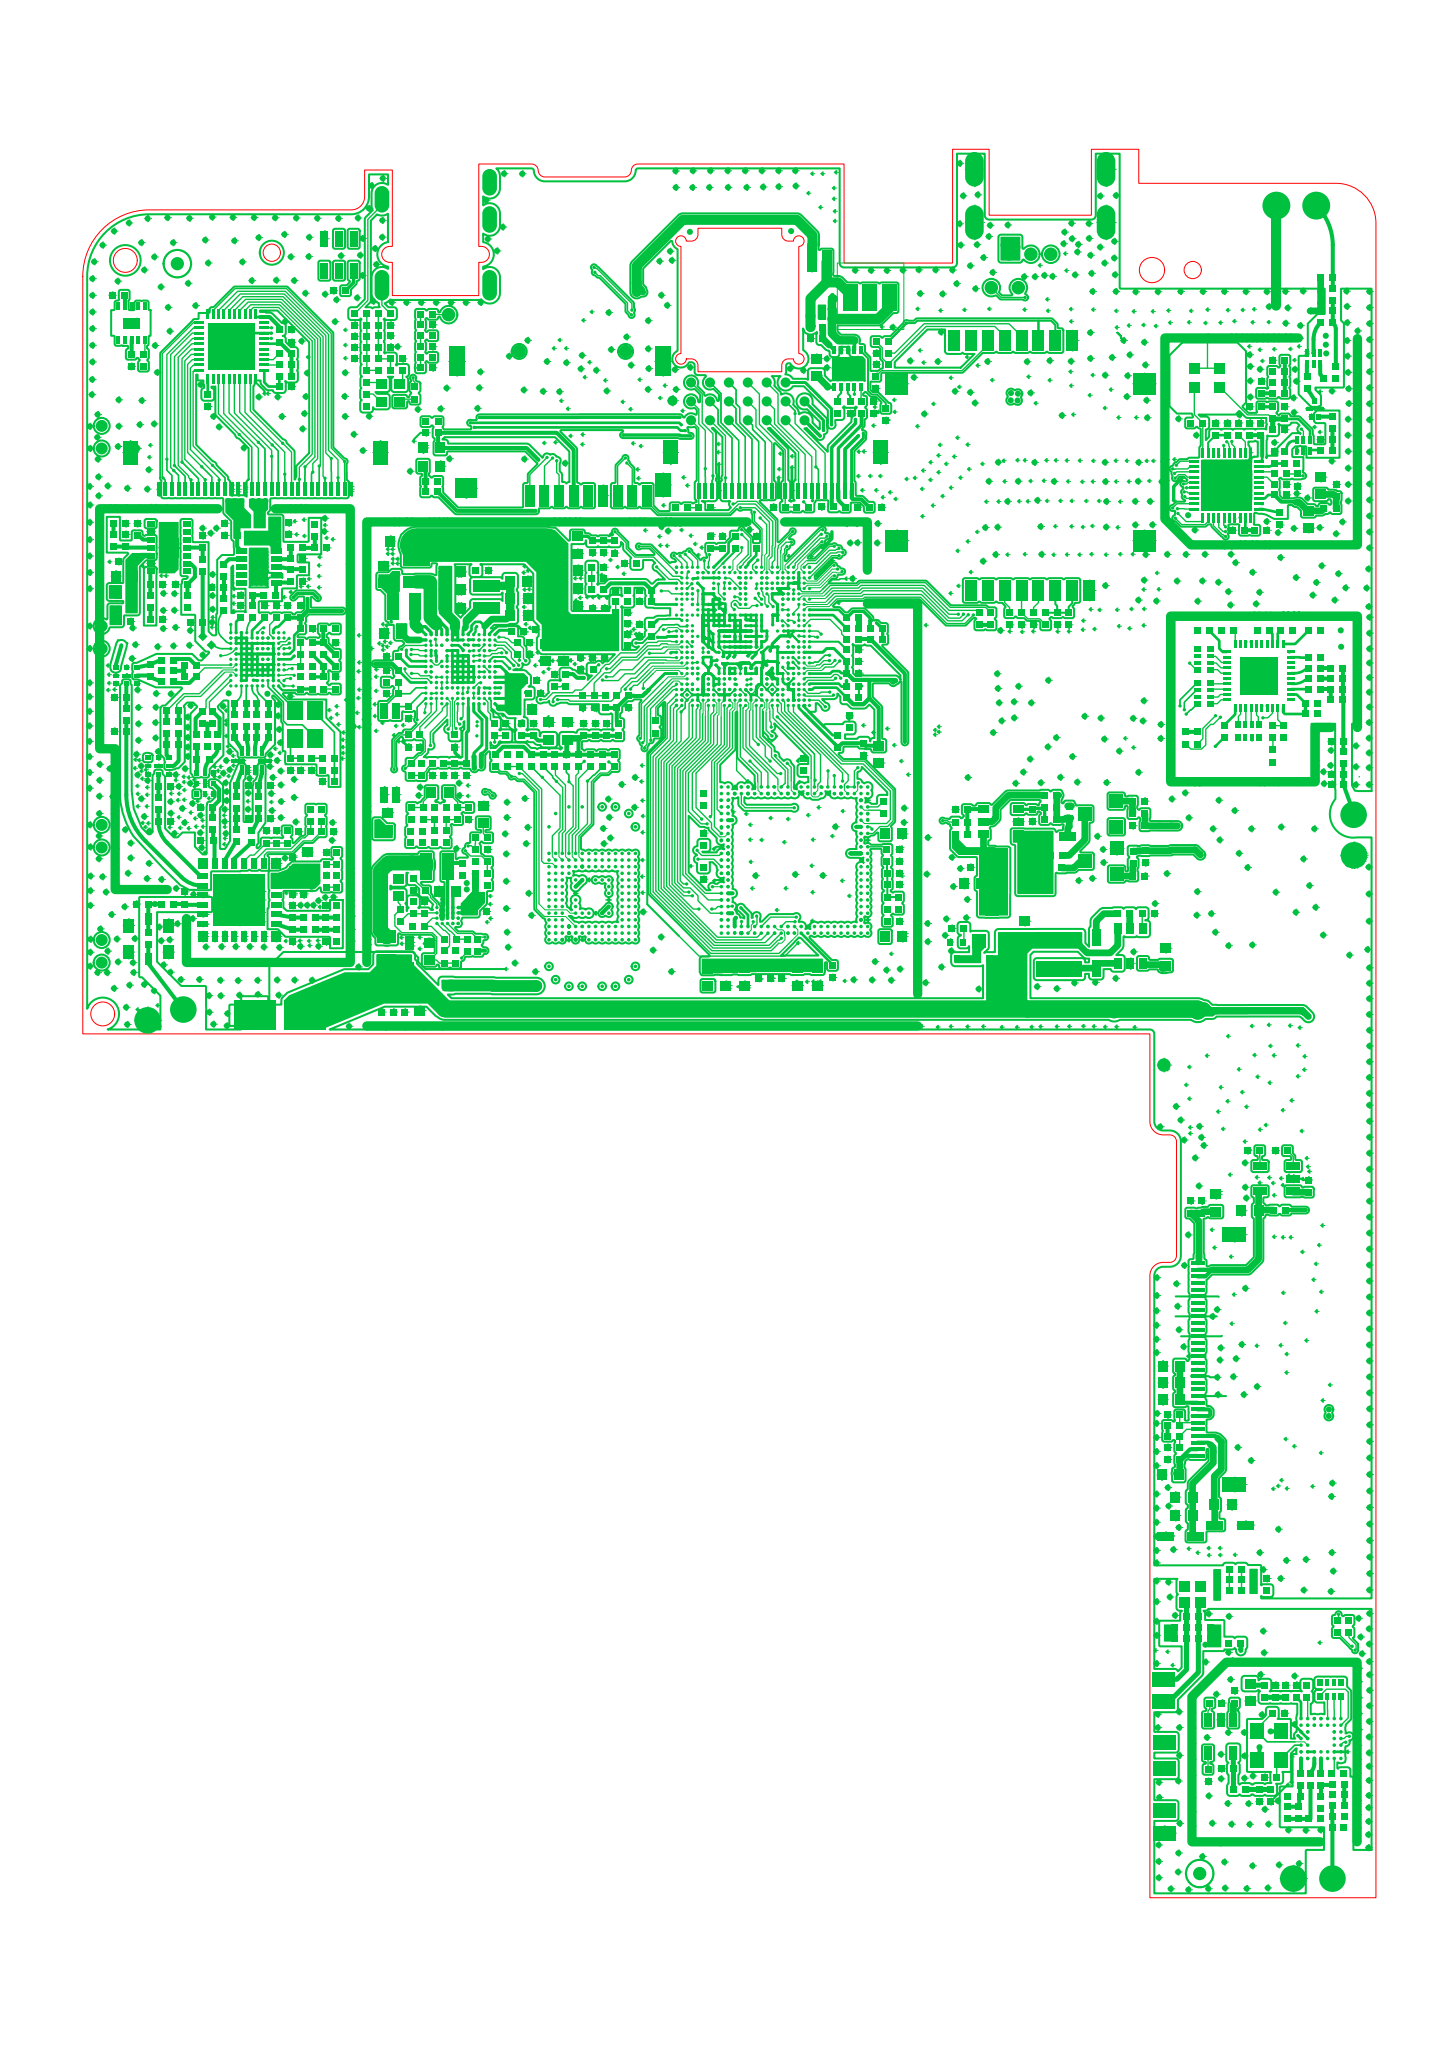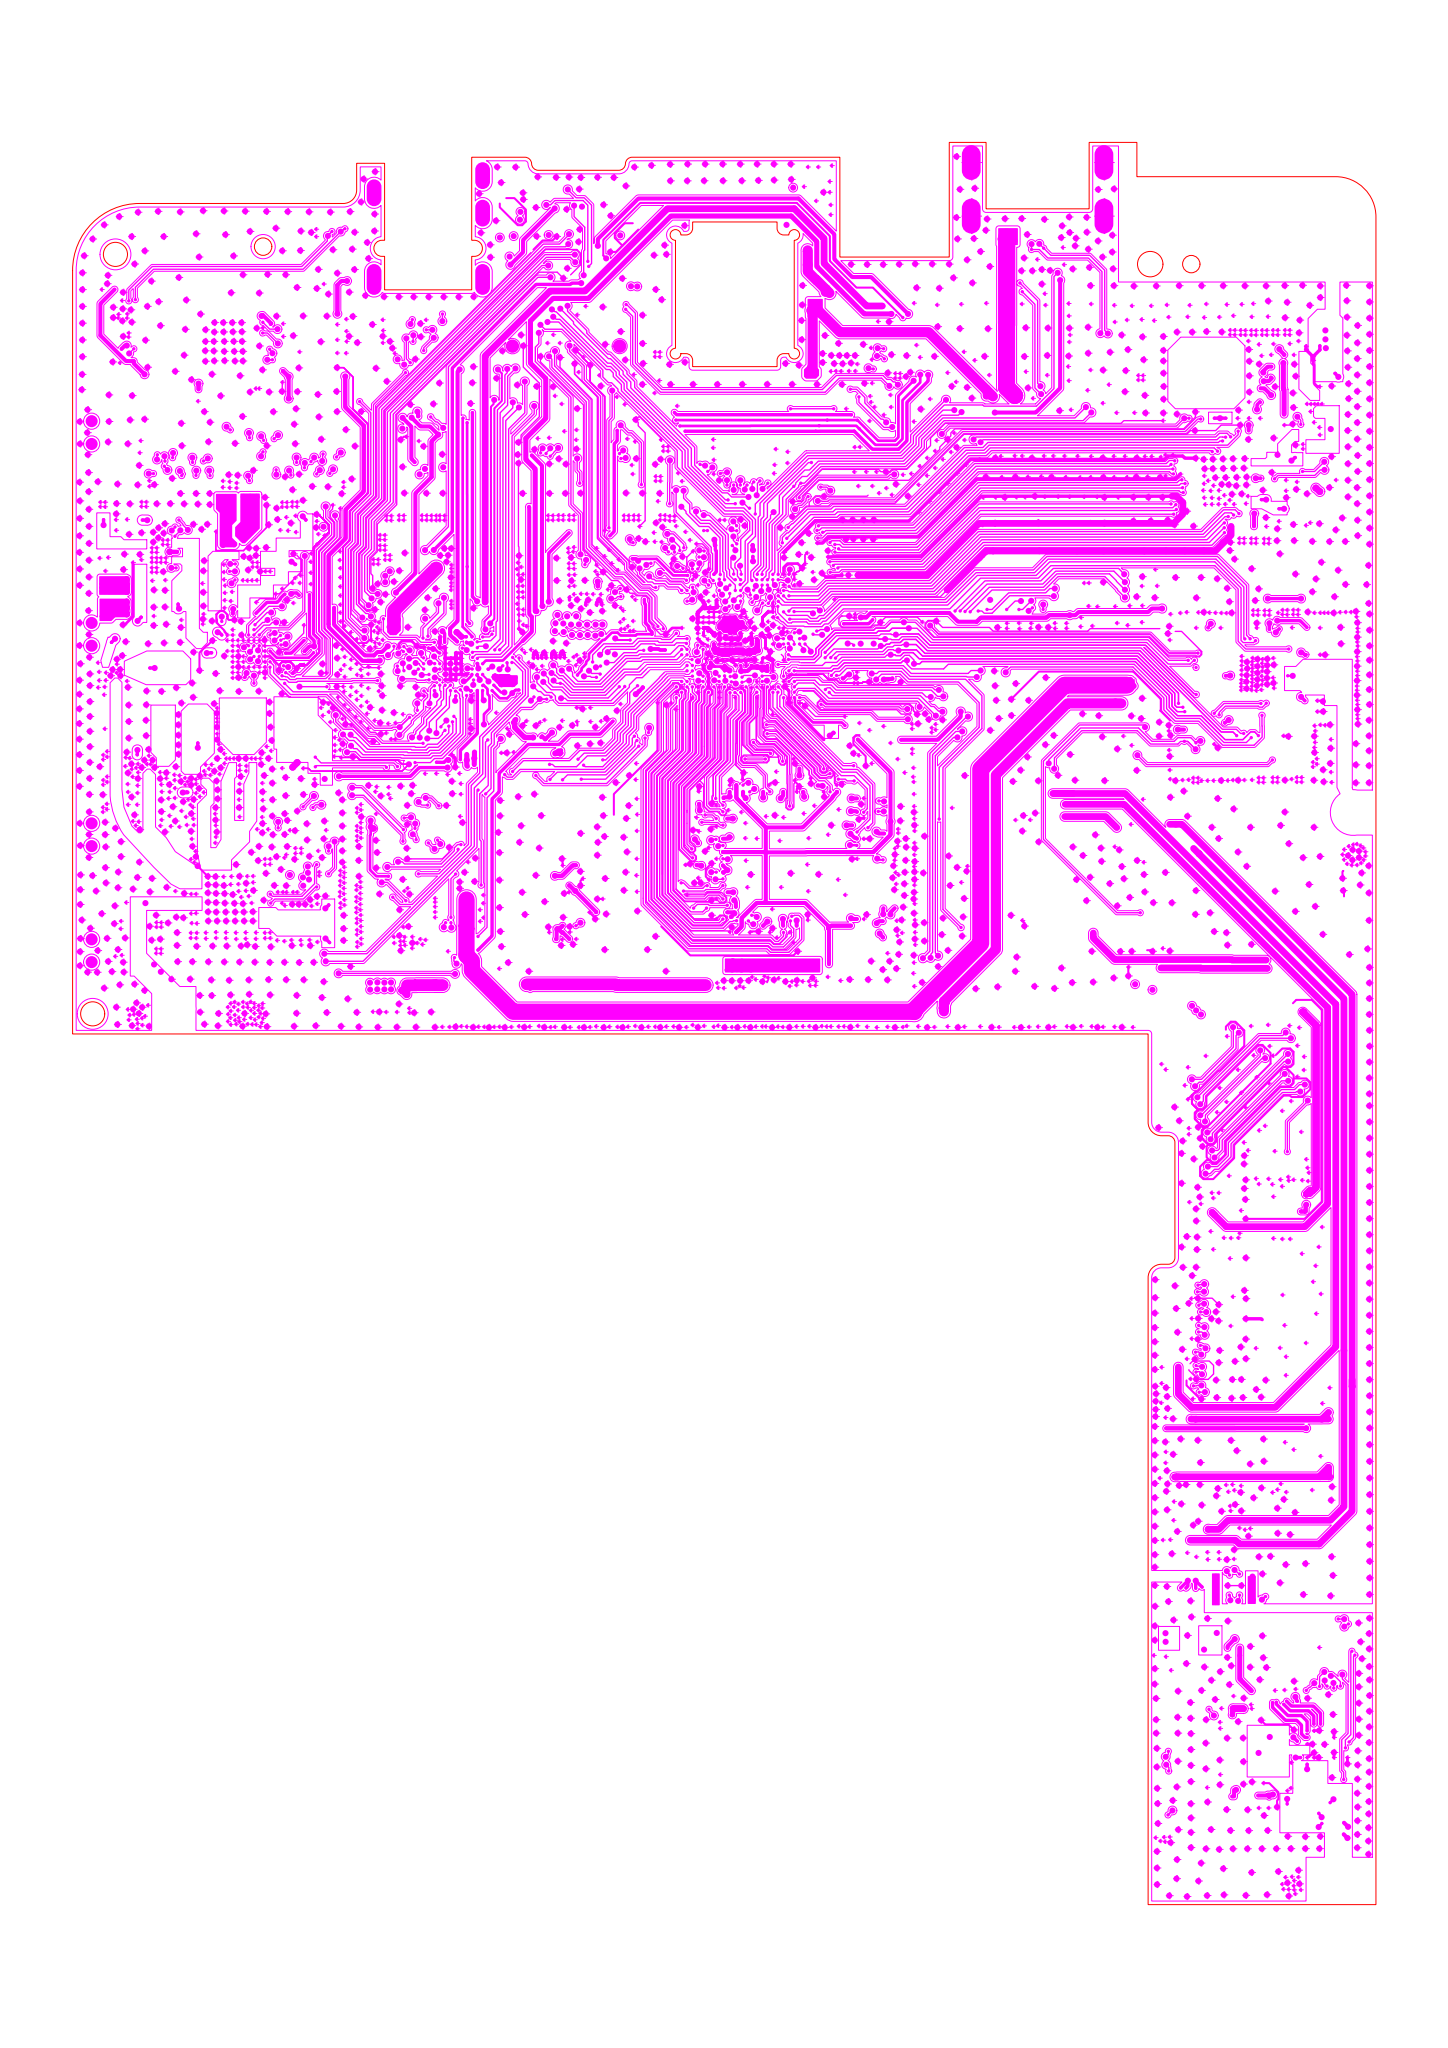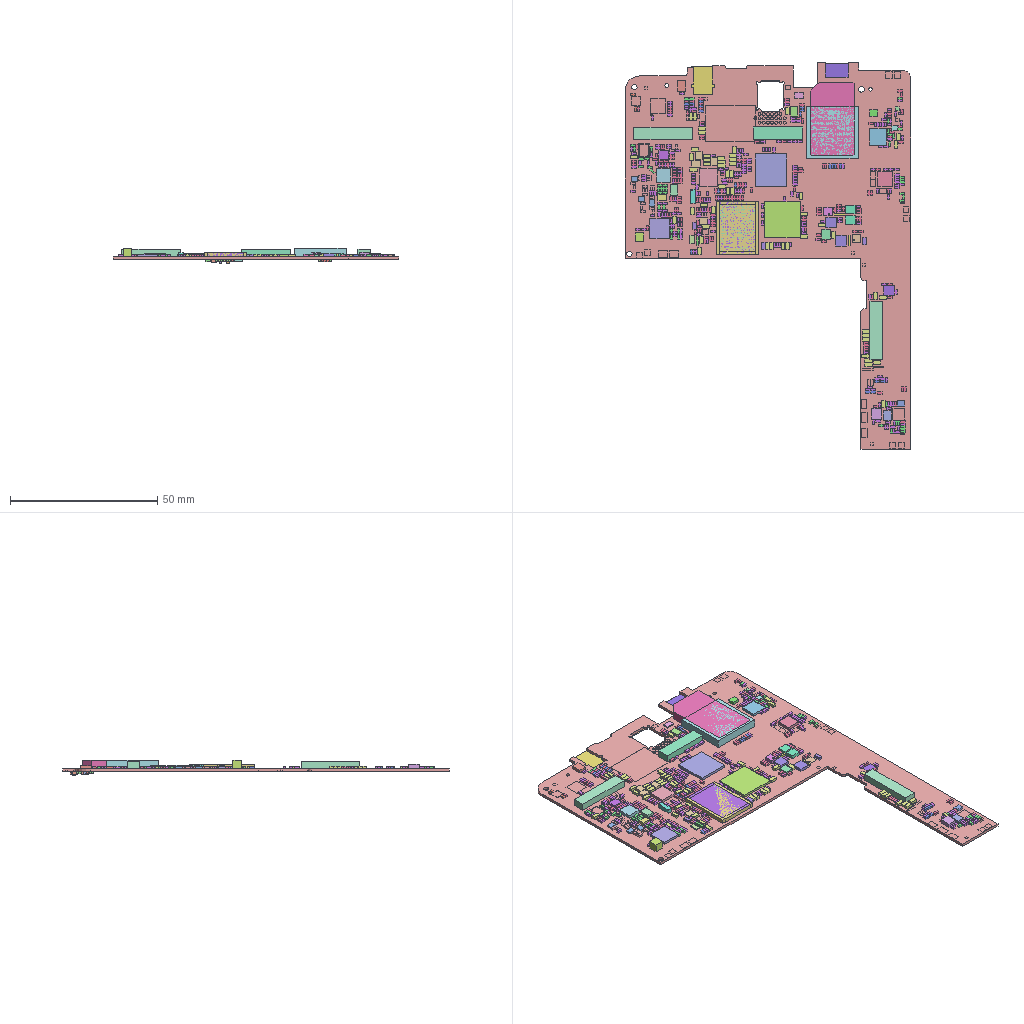Circuit board layout | Siemens PADS | box 97.2 x 131.6 x 5.4 mm
Layer stack:
layer,name,type,plane,layer_thickness_mm,copper_thickness_mm,dielectric_constant
0,,,,0,,1
1,Top,ROUTING,NONE,0.05969,0.03302,4.2
2,Inner Layer 2,ROUTING,NONE,0.2134,0.03302,4.2
3,Inner Layer 3,ROUTING,NONE,0.2108,0.03302,4.2
4,Inner Layer 4,ROUTING,NONE,0.2134,0.03302,4.2
5,Inner Layer 5,ROUTING,NONE,0.05969,0.03302,4.2
6,Bottom,ROUTING,NONE,0,0.03302,1
Part placement, first 531 of 696 lines:
Ref,PartType,Decal,X_mm,Y_mm,Rotation,Layer,Placed,Installed
ANT701,ANTENNA,PAD1-2X3AAA,6.14,-43.067,180,Top,True,True
ANT702,ANTENNA,PAD1-2X3BA,3.451,-43.878,180,Top,True,True
ANT902,ANTENNA,PAD1-2X3C,88.341,17.424,0,Top,True,True
ANT903,ANTENNA,PAD1-2X3C,91.338,17.424,0,Top,True,True
ANT1301,RT_TVPAD_R7210,RT_TVPAD_R7210AAA,94.177,-31.459,0,Top,True,True
ANT1302,RT_TVPAD_R7210,RT_TVPAD_R7210AAA,94.151,-28.411,0,Top,True,True
ANT1303,RT_TVPAD_R7210,RT_TVPAD_R7210B,92.558,-108.458,0,Top,True,True
ANT1304,RT_TVPAD_R7210,RT_TVPAD_R7210B,89.611,-108.458,0,Top,True,True
BAT+,BATCON/4P_1,ANTENNA3X2,15.305,-43.469,90,Top,True,True
BAT-,BATCON/4P_1,ANTENNA3X2,11.514,-43.469,90,Top,True,True
C1,C0603,C0603,48.337,-40.615,270,Top,True,True
C104,C0402,C0402,39.116,-13.208,180,Top,True,True
C108,C0402,C0402,39.776,-9.5,180,Top,True,True
C109,C0402,C0402,46.66,-7.899,90,Top,True,True
C110,C0402,C0402,55.372,-22.885,90,Top,True,True
C111,C0402,C0402,56.49,-17.755,0,Top,True,True
C112,C0402,C0402,45.796,-7.899,90,Top,True,True
C113,C0402,C0402,56.49,-16.866,0,Top,True,True
C115,C0402,C0402,56.49,-18.771,180,Top,True,True
C116,C0402,C0402,56.49,-14.402,180,Top,True,True
C117,C0402,C0402,40.894,-11.506,0,Top,True,True
C119,C0402,C0402,40.869,-14.986,180,Top,True,True
C120,C0402,C0402,40.869,-14.072,180,Top,True,True
C122,C0402,C0402,56.49,-13.589,180,Top,True,True
C123,C0402,C0402,49.228,-7.922,270,Top,True,True
C124,C0402,C0402,39.116,-15.697,180,Top,True,True
C125,C0402,C0402,39.599,-19.914,90,Top,True,True
C127,C0402,C0402,40.894,-12.344,0,Top,True,True
C128,C0402,C0402,56.49,-19.609,180,Top,True,True
C129,C0603,C0603,35.154,-11.405,0,Top,True,True
C130,C0603,C0603,46.94,-40.615,270,Top,True,True
C131,C0402,C0402,37.795,-13.31,270,Top,True,True
C132,C0603,C0603,33.361,-16.184,270,Top,True,True
C133,C0603,C0603,35.155,-10.016,0,Top,True,True
C134,C0603,C0603,35.154,-12.751,0,Top,True,True
C136,C0603,C0603,34.739,-16.181,270,Top,True,True
C140,C0402,C0402,36.932,-13.31,270,Top,True,True
C142,C0402,C0402,51.16,-40.269,90,Top,True,True
C143,C0402,C0402,59.54,-36.43,180,Top,True,True
C144,C0402,C0402,49.417,-40.264,90,Top,True,True
C148,C0402,C0402,37.795,-16.154,90,Top,True,True
C151,C0402,C0402,50.332,-40.264,90,Top,True,True
C152,C0402,C0402,36.932,-16.154,90,Top,True,True
C155,C0402,C0402,36.043,-16.154,90,Top,True,True
C156,C0402,C0402,39.116,-14.046,180,Top,True,True
C157,C0402,C0402,39.116,-14.859,180,Top,True,True
C158,C0402,C0402,33.096,-14.478,0,Top,True,True
C201,C0402,C0402,37.313,-9.779,180,Top,True,True
C208,R0402,R0402,37.033,-19.914,90,Top,True,True
C213,C0402,C0402,47.65,-7.899,90,Top,True,True
C219,C0402,C0402,86.792,2.286,180,Top,True,True
C221,C0402,C0402,87.178,-7.001,0,Top,True,True
C225,C0402,C0402,85.476,-7.001,180,Top,True,True
C241,C0402,C0402,26.568,-22.86,90,Top,True,True
C242,C0402,C0402,26.568,-24.994,90,Top,True,True
C243,C0402,C0402,25.705,-24.994,90,Top,True,True
C301,C0603,C0603,26.365,-11.481,0,Top,True,True
C302,C0603,C0603,21.869,-14.757,180,Top,True,True
C303,C0603,C0603,26.365,-12.852,0,Top,True,True
C304,C0402,C0402,32.258,-18.288,180,Top,True,True
C306,C0603,C0603,31.377,-12.14,0,Top,True,True
C307,C0402,C0402,21.869,-16.485,0,Top,True,True
C308,C0402,C0402,21.869,-17.551,0,Top,True,True
C309,C0603,C0603,26.365,-10.135,0,Top,True,True
C311,C0603,C0603,31.377,-13.41,0,Top,True,True
C314,C0603,C0603,23.927,-42.494,270,Top,True,True
C316,C0402,C0402,31.75,-15.469,180,Top,True,True
C317,R0402,R0402,31.75,-16.332,180,Top,True,True
C318,C0402,C0402,28.569,-31.028,180,Top,True,True
C319,C0402,C0402,23.063,-20.726,90,Top,True,True
C320,C0402,C0402,31.293,-14.656,180,Top,True,True
C321,C0402,C0402,23.927,-22.86,270,Top,True,True
C322,C0402,C0402,23.063,-22.86,270,Top,True,True
C323,C0402,C0402,27.432,-24.994,90,Top,True,True
C324,C0402,C0402,21.869,-19.304,0,Top,True,True
C329,C0402,C0402,22.8,-42.8,90,Top,True,True
C330,C0402,C0402,32.537,-19.253,180,Top,True,True
C331,C0402,C0402,87.63,-86.335,270,Top,True,True
C333,C0603,C0603,22.352,-7.823,180,Top,True,True
C334,C0603,C0603,21.209,-10.338,90,Top,True,True
C335,C0603,C0603,31.369,-10.846,0,Top,True,True
C336,C0603,C0603,31.674,-20.472,0,Top,True,True
C341,C0603,C0603,21.488,-28.905,90,Top,True,True
C356,C0603,C0603,28.695,-28.386,90,Top,True,True
C401,C0402,C0402,23.8,-36.805,0,Top,True,True
C403,C0402,C0402,52.809,-24.619,90,Top,True,True
C405,C0603,C0603,25.998,-34.185,180,Top,True,True
C407,C0402,C0402,23.901,-34.138,0,Top,True,True
C408,C0603,C0603,24.638,-38.684,90,Top,True,True
C409,C0402,C0402,28.473,-35.687,180,Top,True,True
C410,C0402,C0402,27.16,-32.498,90,Top,True,True
C417,C0402,C0402,26.619,-39.116,270,Top,True,True
C420,C0402,C0402,21.26,6.782,0,Top,True,True
C422,C0402,C0402,19.482,6.756,180,Top,True,True
C500,C0402,C0402,86.177,-85.96,180,Top,True,True
C502,C0402,C0402,82.956,-89.586,0,Top,True,True
C503,C0402,C0402,81.128,-89.586,0,Top,True,True
C505,C0603,C0603,25.451,-26.746,0,Top,True,True
C506,C0402,C0402,85.263,-85.172,0,Top,True,True
C507,C0402,C0402,25.908,-28.321,270,Top,True,True
C508,C0402,C0402,25.019,-28.321,270,Top,True,True
C510,C0402,C0402,38.297,13.93,270,Bottom,True,True
C511,C0402,C0402,38.297,15.647,90,Bottom,True,True
C512,C0402,C0402,37.434,14.732,270,Bottom,True,True
C521,C0402,C0402,82.042,-88.773,0,Top,True,True
C522,C0402,C0402,19.482,5.918,0,Top,True,True
C523,C0402,C0402,20.828,5.486,90,Top,True,True
C524,C0402,C0402,22.174,5.893,0,Top,True,True
C525,C0402,C0402,23.685,-29.669,180,Top,True,True
C526,C0402,C0402,34.715,13.778,270,Bottom,True,True
C530,C0603,C0603,21.031,3.327,270,Top,True,True
C531,C0603,C0603,22.413,3.328,270,Top,True,True
C532,C0603,C0603,32.734,14.032,90,Bottom,True,True
C533,C0402,C0402,34.69,11.975,270,Bottom,True,True
C534,C0402,C0402,36.468,12.838,270,Bottom,True,True
C535,C0402,C0402,23.685,-30.507,180,Top,True,True
C599,C0402,C0402,84.348,-85.96,180,Top,True,True
C601,C0603,C0603,59.565,-37.577,180,Top,True,True
C603,C0402,C0402,57.296,-23.484,270,Top,True,True
C604,C0603,C0603,58.439,-23.865,270,Top,True,True
C605,C0402,C0402,45.285,-27.243,90,Top,True,True
C606,C0402,C0402,45.256,-32.806,270,Top,True,True
C607,C0603,C0603,59.565,-29.852,180,Top,True,True
C608,C0402,C0402,54.959,-40.2,270,Top,True,True
C610,R0402,R0402,6.248,-34.671,270,Top,True,True
C611,C0603,C0603,52.308,-40.611,270,Top,True,True
C612,C0603,C0603,53.806,-40.611,270,Top,True,True
C613,C0402,C0402,45.285,-30.247,270,Top,True,True
C615,C0402,C0402,59.083,-35.059,270,Top,True,True
C616,C0402,C0402,59.54,-33.662,180,Top,True,True
C617,C0402,C0402,59.54,-32.823,180,Top,True,True
C629,C0402,C0402,30.499,-24.322,90,Top,True,True
C630,C0402,C0402,31.388,-24.322,90,Top,True,True
C644,C0603,C0603,35.045,-22.112,90,Top,True,True
C645,C0402,C0402,36.214,-22.01,90,Top,True,True
C646,C0402,C0402,37.103,-22.01,90,Top,True,True
C651,C0603,C0603,33.623,-22.112,90,Top,True,True
C652,C0402,C0402,37.992,-22.01,90,Top,True,True
C655,C0402,C0402,32.455,-22.01,90,Top,True,True
C701,C0402,C0402,12.268,-26.213,180,Top,True,True
C702,C0402,C0402,12.268,-28.702,180,Top,True,True
C703,C0402,C0402,10.566,-28.702,180,Top,True,True
C705,C0402,C0402,15.418,-14.427,0,Top,True,True
C706,C0402,C0402,10.566,-26.213,180,Top,True,True
C708,C0402,C0402,11.252,-30.074,270,Top,True,True
C709,C0402,C0402,10.109,-29.947,270,Top,True,True
C713,C0402,C0402,17.12,-15.469,180,Top,True,True
C714,C0402,C0402,14.963,-13.125,270,Top,True,True
C726,C0402,C0402,13.945,-13.132,270,Top,True,True
C727,C0402,C0402,14.961,-18.491,270,Top,True,True
C733,C0402,C0402,15.189,-33.985,90,Top,True,True
C736,C0402,C0402,14.376,-33.985,90,Top,True,True
C737,C0402,C0402,12.268,-13.132,90,Top,True,True
C738,C0402,C0402,14.376,-32.08,270,Top,True,True
C745,C0402,C0402,10.414,-13.132,270,Top,True,True
C747,C0402,C0402,4.978,-35.128,0,Top,True,True
C754,C0402,C0402,15.773,-24.613,90,Top,True,True
C757,C0603,C0603,15.443,-31.877,90,Top,True,True
C771,C0402,C0402,15.621,-36.144,0,Top,True,True
C773,C0402,C0402,17.653,-37.516,270,Top,True,True
C774,C0402,C0402,17.653,-35.687,90,Top,True,True
C778,C0402,C0402,15.621,-37.059,0,Top,True,True
C781,C0402,C0402,12.365,-30.079,270,Top,True,True
C783,C0402,C0402,15.265,-29.693,180,Top,True,True
C785,C0402,C0402,3.048,-35.128,180,Top,True,True
C793,C0402,C0402,16.967,-29.693,0,Top,True,True
C798,C0402,C0402,16.891,-31.699,90,Top,True,True
C799,C0402,C0402,16.891,-33.401,90,Top,True,True
C805,C0402,C0402,13.614,-6.452,180,Top,True,True
C809,C0402,C0402,1.238,10.679,180,Top,True,True
C810,C0402,C0402,2.227,5.782,270,Top,True,True
C812,C0402,C0402,14.681,-9.119,180,Top,True,True
C815,C0402,C0402,16.485,-8.331,180,Top,True,True
C819,C0603,C0603,1.7,-10.454,0,Top,True,True
C825,C0603,C0603,33.29,17.82,90,Bottom,True,True
C827,C0402,C0402,6.452,-12.344,270,Top,True,True
C828,C0402,C0402,1.71,-13.868,180,Top,True,True
C829,C0402,C0402,3.658,-12.37,90,Top,True,True
C830,C0402,C0402,7.595,-9.677,270,Top,True,True
C831,C0402,C0402,1.713,-9.355,180,Top,True,True
C832,C0402,C0402,0.889,-7.772,270,Top,True,True
C834,C0402,C0402,4.928,-18.364,0,Top,True,True
C838,C0402,C0402,4.928,-16.789,0,Top,True,True
C839,C0402,C0402,4.928,-17.577,0,Top,True,True
C852,C0402,C0402,1.397,-22.123,180,Top,True,True
C862,C0402,C0402,13.614,-7.29,180,Top,True,True
C863,C0402,C0402,9.728,-6.477,0,Top,True,True
C864,C0402,C0402,9.728,-7.391,0,Top,True,True
C865,C0402,C0402,9.195,-12.598,270,Top,True,True
C873,C0402,C0402,7.95,-22.835,90,Top,True,True
C874,C0402,C0402,8.738,-22.835,90,Top,True,True
C876,C0402,C0402,7.163,-22.835,90,Top,True,True
C877,C0402,C0402,7.925,-30.353,180,Top,True,True
C903,C0402,C0402,21.937,-42.8,90,Top,True,True
C913,C0402,C0402,84.647,-100.196,180,Top,True,True
C927,C0603,C0603,91.669,-3.658,270,Top,True,True
C933,C0402,C0402,92.354,4.42,180,Top,True,True
C934,C0402,C0402,87.224,3.759,90,Top,True,True
C936,C0402,C0402,87.173,0.6096,90,Top,True,True
C937,C0402,C0402,92.558,1.092,270,Top,True,True
C943,C0402,C0402,92.837,-4.013,90,Top,True,True
C944,C0402,C0402,90.653,4.089,90,Top,True,True
C950,R0402,R0402,92.1,-0.1778,0,Top,True,True
C951,C0402,C0402,88.519,0.5588,0,Top,True,True
C952,C0402,C0402,88.976,1.829,90,Top,True,True
C954,C0402,C0402,84.633,0.6096,270,Top,True,True
C956,C0402,C0402,88.519,5.791,180,Top,True,True
C957,C0402,C0402,86.335,0.6096,270,Top,True,True
C958,C0402,C0402,85.496,0.6096,270,Top,True,True
C963,C0402,C0402,83.769,0.6096,270,Top,True,True
C972,R0402,R0402,92.126,11.989,0,Top,True,True
C1006,C0402,C0402,80.613,-76.925,0,Top,True,True
C1008,C0402,C0402,81.902,-57.925,270,Top,True,True
C1010,C0603,C0603,80.435,-72.43,180,Top,True,True
C1017,C0603,C0603,80.435,-69.89,0,Top,True,True
C1022,C0402,C0402,86.633,-53.684,180,Top,True,True
C1023,C0603,C0603,90.752,-6.196,90,Top,True,True
C1024,C0603,C0603,69.412,-37.073,270,Top,True,True
C1029,C0402,C0402,88.646,-4.343,0,Top,True,True
C1031,C0603,C0603,86.353,-58.206,180,Top,True,True
C1034,C0603,C0603,80.435,-71.16,0,Top,True,True
C1040,C0603,C0603,83.788,-57.621,90,Top,True,True
C1042,C0402,C0402,71.778,-31.473,180,Top,True,True
C1044,C0402,C0402,77.975,-27.384,0,Top,True,True
C1046,C0603,C0603,81.384,-79.751,0,Top,True,True
C1048,C0603,C0603,81.391,-81.139,0,Top,True,True
C1049,C0402,C0402,78.001,-33.022,0,Top,True,True
C1050,C0402,C0402,71.752,-32.413,180,Top,True,True
C1052,C0603,C0603,84.321,-80.329,180,Top,True,True
C1055,C0603,C0603,80.354,-78.084,0,Top,True,True
C1058,C0402,C0402,71.367,-28.767,0,Top,True,True
C1070,C0603,C0603,65.504,-33.581,0,Top,True,True
C1078,C0402,C0402,65.783,-32.362,0,Top,True,True
C1079,C0402,C0402,90.748,-56.351,270,Top,True,True
C1101,C0603,C0603,24.816,-2.184,180,Top,True,True
C1105,C0402,C0402,13.818,3.81,0,Top,True,True
C1106,C0402,C0402,7.976,2.769,270,Top,True,True
C1107,C0402,C0402,13.818,8.103,0,Top,True,True
C1124,C0402,C0402,13.818,7.137,0,Top,True,True
C1204,C0402,C0402,54.578,-5.247,180,Top,True,True
C1207,C0402,C0402,55.829,1.778,0,Top,True,True
C1208,C0603,C0603,35.773,-8.11,270,Top,True,True
C1209,C0402,C0402,36.906,-8.255,270,Top,True,True
C1212,C0402,C0402,50.952,-5.258,0,Top,True,True
C1219,C0402,C0402,58.185,-5.272,180,Top,True,True
C1220,C0402,C0402,56.381,-5.272,180,Top,True,True
C1221,C0402,C0402,38.577,-8.257,90,Top,True,True
C1222,C0402,C0402,37.75,-8.249,90,Top,True,True
C1223,C0402,C0402,45.364,-5.309,180,Top,True,True
C1235,C0603,C0603,53.746,5.258,90,Top,True,True
C1236,C0402,C0402,55.829,2.692,180,Top,True,True
C1237,C0402,C0402,53.772,7.417,0,Top,True,True
C1260,C0402,C0402,57.603,1.779,0,Top,True,True
C1262,C0402,C0402,28.6,-10.033,0,Top,True,True
C1301,C0402,C0402,87.909,-100.838,180,Top,True,True
C1302,C0402,C0402,88.494,-96.012,0,Top,True,True
C1303,C0402,C0402,89.052,-94.361,90,Top,True,True
C1304,C0402,C0402,87.376,-14.579,180,Top,True,True
C1305,C0402,C0402,87.912,-102.206,270,Top,True,True
C1306,C0402,C0402,90.119,-101.016,90,Top,True,True
C1307,C0402,C0402,91.237,-103.962,0,Top,True,True
C1308,C0402,C0402,92.888,-19.736,180,Top,True,True
C1309,C0402,C0402,89.992,-103.505,90,Top,True,True
C1310,C0402,C0402,89.84,-94.361,90,Top,True,True
C1311,C0402,C0402,85.192,-94.793,90,Top,True,True
C1312,C0402,C0402,89.662,-102.26,180,Top,True,True
C1314,C0402,C0402,82.855,-14.579,180,Top,True,True
C1316,C0603,C0603,86.36,-94.437,90,Top,True,True
C1317,C0402,C0402,87.036,-102.208,270,Top,True,True
C1318,C0402,C0402,88.265,-94.361,90,Top,True,True
C1319,C0402,C0402,91.694,-102.718,270,Top,True,True
C1320,C0402,C0402,88.055,-23.992,90,Top,True,True
C1321,C0402,C0402,91.186,-14.579,0,Top,True,True
C1322,C0402,C0402,91.186,-16.586,0,Top,True,True
C1323,C0402,C0402,91.186,-18.948,180,Top,True,True
C1324,C0402,C0402,91.186,-18.161,180,Top,True,True
C1325,C0402,C0402,91.186,-17.373,180,Top,True,True
C1326,C0402,C0402,89.078,-14.579,0,Top,True,True
C1327,C0402,C0402,92.989,-101.346,180,Top,True,True
C1328,C0402,C0402,90.983,-20.828,0,Top,True,True
C1329,C0402,C0402,90.983,-20.015,0,Top,True,True
C1330,C0402,C0402,88.893,-22.163,270,Top,True,True
C1332,C0402,C0402,84.404,-22.149,270,Top,True,True
C1338,C0402,C0402,83.201,-100.692,270,Top,True,True
C1401,C0402,C0402,17.882,11.024,180,Top,True,True
C1502,C0603,C0603,24.816,-0.8128,180,Top,True,True
C1507,C0402,C0402,24.841,0.3302,180,Top,True,True
C1601,C0402,C0402,38.307,11.902,90,Bottom,True,True
C1602,C0402,C0402,72.72,-13.665,90,Top,True,True
CON402,J_,USB_5PINA,70.582,22.11,180,Bottom,False,True
CON421,RF-CON,RF-CON,3.505,-37.744,180,Top,True,True
CON801,SIMYS-3016S1-TP00,SIMYS-3016S1-TP00,69.088,-2.134,180,Top,False,True
CON1001,30PIN,CON30-0.5,82.41,-70.402,90,Top,True,True
CON1201,2PIN,VIB_X560,53.975,13.233,180,Top,True,True
CON1401,30PIN,CON30-0.5,12.529,-3.92,180,Top,True,True
CON1402,MMC_CONN_0,TF_CARD1,42.199,6.052,180,Top,True,True
D6,DIODE/ZENER,SOD-523(PZ5D4V2H),23.172,-39.027,270,Top,True,True
D402,WSB5503W-SOD323,SOD-323,66.37,13.792,90,Bottom,True,True
D501,T0402,T0402,31.166,18.491,180,Bottom,True,True
D1001,DIODE_ZENER_LL34,SOD-323,81.146,-82.691,270,Top,True,True
D1002,DIODE_ZENER_LL34,SOD-323AA,84.855,-81.853,270,Top,True,True
D1004,DIODE_SCHOTTKY_6,SOD323,71.498,-30.051,90,Top,True,True
D1005,DIODE_SCHOTTKY_6,SOD323,74.796,-38.8,180,Top,True,True
FB1301,L0402,L0402,85.573,-101.752,0,Top,True,True
FB1302,L0402,L0402,87.478,-94.361,270,Top,True,True
J501,Y-J3CQ5-20WA,Y-J3CQ5-20WA,25.124,20.431,180,Bottom,False,True
J1501,FPC0512-24RL-TAX,CON24-0.5,50.153,-3.917,180,Top,True,True
L301,INDUCTOR,L/IND/SMD/2520,23.647,-10.058,90,Top,True,True
L302,INDUCTOR,L/IND/SMD/2520,22.733,-12.725,180,Top,True,True
L303,INDUCTOR,L/IND/SMD/2520,28.931,-12.014,90,Top,True,True
L402,L0603,L0603,31.344,17.501,180,Bottom,True,True
L403,INDUCTOR,L/IND/SMD/2520,25.222,-32.309,180,Top,True,True
L442,L0402,L0402,7.569,-21.107,90,Top,True,True
L501,L0402,L0402,36.138,15.19,0,Bottom,True,True
L503,L0402,L0402,25.019,-30.074,90,Top,True,True
L504,L0402,L0402,25.908,-30.074,90,Top,True,True
L505,L0402,L0402,30.99,14.006,180,Bottom,True,True
L506,L0402,L0402,19.482,9.296,0,Top,True,True
L507,L0402,L0402,21.26,9.296,180,Top,True,True
L509,L0402,L0402,36.138,14.275,0,Bottom,True,True
L510,L0402,L0402,19.922,2.791,270,Top,True,True
L512,L0603,L0603,81.458,-87.071,270,Top,True,True
L513,L0603,L0603,82.613,-87.071,270,Top,True,True
L517,L0402,L0402,23.561,3.32,90,Top,True,True
L630,L0402,L0402,7.925,-15.316,135,Top,True,True
L700,L0402,L0402,9.957,-21.336,90,Top,True,True
L701,L0402,L0402,16.866,-37.516,90,Top,True,True
L703,L0402,L0402,14.376,-37.516,90,Top,True,True
L704,L0402,L0402,16.866,-35.687,270,Top,True,True
L705,L0402,L0402,14.376,-35.687,270,Top,True,True
L707,L0402,L0402,11.811,-27.457,90,Top,True,True
L708,L0402,L0402,10.109,-27.457,90,Top,True,True
L715,L0402,L0402,10.414,-22.606,0,Top,True,True
L716,L0402,L0402,10.414,-20.066,0,Top,True,True
L719,L0402,L0402,10.871,-21.336,90,Top,True,True
L723,L0402,L0402,11.659,-21.336,90,Top,True,True
L724,L0402,L0402,12.116,-22.606,0,Top,True,True
L725,L0402,L0402,12.116,-20.066,0,Top,True,True
L726,L0402,L0402,12.573,-21.336,90,Top,True,True
L801,L0402,L0402,8.331,-29.083,270,Top,True,True
L802,L0402,L0402,7.137,-13.97,0,Top,True,True
L804,L0402,L0402,3.658,-17.577,270,Top,True,True
L805,L0402,L0402,7.595,-7.874,270,Top,True,True
L806,L0402,L0402,4.115,-11.1,180,Top,True,True
L809,L0402,L0402,4.13,-13.699,180,Top,True,True
L810,L0402,L0402,5.994,-11.074,0,Top,True,True
L821,L0402,L0402,1.803,-7.772,270,Top,True,True
L822,L0402,L0402,1.346,-6.502,180,Top,True,True
L829,L0402,L0402,6.655,-17.983,0,Top,True,True
L830,L0402,L0402,7.874,-27.838,180,Top,True,True
L833,L0402,L0402,8.357,-21.107,270,Top,True,True
L834,L0402,L0402,7.62,-24.232,180,Top,True,True
L850,L0402,L0402,1.854,-20.853,270,Top,True,True
L851,L0402,L0402,1.397,-19.583,180,Top,True,True
L852,L0402,L0402,4.726,-28.904,180,Top,True,True
L853,L0402,L0402,6.655,-17.196,180,Top,True,True
L855,L0402,L0402,16.025,-6.994,90,Top,True,True
L856,L0402,L0402,4.877,-21.869,270,Top,True,True
L857,L0402,L0402,5.791,-21.869,270,Top,True,True
L858,L0402,L0402,5.334,-23.114,180,Top,True,True
L859,L0402,L0402,5.334,-20.599,180,Top,True,True
L860,L0402,L0402,4.724,-26.314,180,Top,True,True
L861,L0402,L0402,4.267,-27.559,90,Top,True,True
L877,L0402,L0402,14.681,-8.331,0,Top,True,True
L906,L0402,L0402,92.913,-22.911,0,Top,True,True
L910,L0402,L0402,88.189,-1.524,90,Top,True,True
L911,L0402,L0402,92.126,9.5,180,Top,True,True
L912,L0402,L0402,88.062,1.829,270,Top,True,True
L948,L0402,L0402,92.1,-0.9652,180,Top,True,True
L949,L0402,L0402,89.916,-3.226,270,Top,True,True
L955,L0402,L0402,88.646,-2.769,180,Top,True,True
L1001,L3030,L3030,68.679,-32.667,90,Top,True,True
L1002,L3030,L3030,72.028,-38.927,180,Top,True,True
L1007,L0402,L0402,88.595,-6.147,270,Top,True,True
L1301,L0402,L0402,90.907,-101.016,90,Top,True,True
L1302,L0402,L0402,91.694,-101.016,90,Top,True,True
L1303,L0402,L0402,89.205,-103.505,90,Top,True,True
L1304,L0402,L0402,93.37,-24.13,90,Top,True,True
L1305,L0402,L0402,92.913,-25.349,0,Top,True,True
L1307,L0402,L0402,92.888,-17.373,180,Top,True,True
L1308,L0402,L0402,92.888,-18.161,180,Top,True,True
L1309,L0402,L0402,92.888,-18.948,180,Top,True,True
L1310,L0402,L0402,92.989,-102.972,0,Top,True,True
L1311,L0402,L0402,92.989,-102.159,0,Top,True,True
L1312,L0402,L0402,92.989,-103.784,180,Top,True,True
LED801,RF-WNIA30DS-EE-F,LED,57.766,10.492,0,Top,True,True
M1,FIDUCIAL_1MM,FIDUCIAL_1MM_A,5.69,13.056,0,Top,True,True
M2,FIDUCIAL_1MM,FIDUCIAL_1MM_A,82.575,-108.077,0,Top,True,True
MIC400,MICROPHONE_2,0805T,79.92,-98.198,0,Top,True,True
NTC201,NTC_/_NCP15WF104F03RC_/_0402_,R0402,37.313,-10.617,0,Top,True,True
Q1001,BAT54S,SOT23,73.937,-28.349,90,Top,True,True
Q1004,BAT54S,SOT23,73.962,-31.905,90,Top,True,True
R51,R0402,R0402,27.61,-28.321,270,Top,True,True
R102,R0603,R0603,45.593,-40.63,90,Top,True,True
R103,R0402,R0402,39.116,-12.344,0,Top,True,True
R104,R0402,R0402,58.279,-15.2,0,Top,True,True
R105,R0402,R0402,58.26,-14.395,0,Top,True,True
R107,R0402,R0402,39.116,-11.506,0,Top,True,True
R201,R0402,R0402,36.5,-17.45,180,Top,True,True
R203,R0402,R0402,56.49,-16.002,0,Top,True,True
R205,R0402,R0402,37.313,-11.481,180,Top,True,True
R206,R0402,R0402,56.49,-15.189,180,Top,True,True
R210,R0402,R0402,82.411,-22.631,270,Top,True,True
R212,R0402,R0402,81.534,-22.631,270,Top,True,True
R217,R0402,R0402,13.818,6.299,180,Top,True,True
R218,R0402,R0402,13.818,5.436,180,Top,True,True
R219,R0402,R0402,66.04,-13.665,90,Top,True,True
R220,R0402,R0402,66.878,-13.665,90,Top,True,True
R221,R0402,R0402,56.221,-21.424,90,Top,True,True
R301,R0402,R0402,34.061,-18.313,90,Top,True,True
R305,R0402,R0402,38.735,-19.914,270,Top,True,True
R309,R0805,R0805,21.438,-38.506,90,Top,True,True
R310,R0603,R0603,22.298,-33.889,270,Top,True,True
R315,R0402,R0402,34.912,-18.279,90,Top,True,True
R316,R0402,R0402,29.534,-22.011,90,Top,True,True
R320,R0402,R0402,23.266,-24.994,270,Top,True,True
R321,R0402,R0402,24.046,-25.009,90,Top,True,True
R322,R0402,R0402,24.866,-25.002,270,Top,True,True
R325,R0402,R0402,28.569,-31.942,180,Top,True,True
R330,R0402,R0402,28.568,-32.856,0,Top,True,True
R333,R0402,R0402,21.858,-18.43,0,Top,True,True
R339,R0402,R0402,28.568,-33.745,0,Top,True,True
R353,R0402,R0402,28.569,-30.139,180,Top,True,True
R406,R0402,R0402,28.296,-38.227,90,Top,True,True
R407,R0402,R0402,19.482,8.433,180,Top,True,True
R408,R0402,R0402,21.26,8.433,0,Top,True,True
R411,R0402,R0402,22.454,-35.992,90,Top,True,True
R412,R0402,R0402,23.419,-32.766,90,Top,True,True
R413,R0402,R0402,24.257,-35.408,90,Top,True,True
R416,R0402,R0402,27.508,-38.227,90,Top,True,True
R419,R0402,R0402,23.444,-35.408,270,Top,True,True
R425,R0402,R0402,26.213,-37.77,180,Top,True,True
R429,R0402,R0402,25.781,-39.116,270,Top,True,True
R454,R0402,R0402,30.99,11.44,0,Bottom,True,True
R456,R0402,R0402,30.99,12.278,0,Bottom,True,True
R504,R0402,R0402,22.174,5.029,0,Top,True,True
R508,R0402,R0402,24.181,-28.321,270,Top,True,True
R514,R0402,R0402,23.317,-28.321,90,Top,True,True
R515,R0402,R0402,35.579,12.838,270,Bottom,True,True
R516,R0402,R0402,33.801,11.975,90,Bottom,True,True
R517,R0402,R0402,33.852,13.778,270,Bottom,True,True
R518,R0402,R0402,31.191,15.697,0,Bottom,True,True
R521,R0402,R0402,31.191,16.535,0,Bottom,True,True
R528,R0402,R0402,26.772,-28.321,90,Top,True,True
R534,R0402,R0402,19.939,4.572,270,Top,True,True
R601,R0402,R0402,34.055,-24.347,90,Top,True,True
R608,R0402,R0402,59.514,-31.02,0,Top,True,True
R609,R0402,R0402,59.921,-35.059,90,Top,True,True
R611,R0402,R0402,59.514,-31.909,0,Top,True,True
R620,R0402,R0402,35.858,-24.347,90,Top,True,True
R621,R0402,R0402,37.662,-24.347,90,Top,True,True
R622,R0402,R0402,32.302,-24.322,90,Top,True,True
R623,R0402,R0402,33.191,-24.322,90,Top,True,True
R624,R0402,R0402,34.944,-24.347,90,Top,True,True
R625,R0402,R0402,36.747,-24.347,90,Top,True,True
R626,R0402,R0402,38.551,-24.322,90,Top,True,True
R627,R0402,R0402,29.61,-24.322,270,Top,True,True
R636,R0402,R0402,31.566,-22.011,90,Top,True,True
R643,R0402,R0402,38.881,-22.011,90,Top,True,True
R645,R0402,R0402,58.794,-27.853,270,Top,True,True
R675,R0402,R0402,41.675,-21.807,90,Top,True,True
R702,R0402,R0402,15.418,-17.247,180,Top,True,True
R703,R0402,R0402,17.12,-14.427,180,Top,True,True
R705,R0402,R0402,15.418,-15.469,180,Top,True,True
R708,R0402,R0402,17.577,-16.789,270,Top,True,True
R714,R0402,R0402,13.157,-13.132,90,Top,True,True
R720,R0402,R0402,14.986,-24.613,270,Top,True,True
R738,R0402,R0402,16.662,-16.789,90,Top,True,True
R741,R0402,R0402,17.577,-18.491,270,Top,True,True
R743,R0402,R0402,16.662,-18.491,270,Top,True,True
R744,R0402,R0402,17.678,-31.699,270,Top,True,True
R746,R0402,R0402,15.875,-18.491,270,Top,True,True
R752,R0402,R0402,17.678,-33.401,270,Top,True,True
R755,R0402,R0402,3.503,-37.745,270,Top,True,True
R756,R0402,R0402,11.379,-13.132,90,Top,True,True
R758,R0402,R0402,12.649,-11.887,0,Top,True,True
R759,R0402,R0402,16.51,-28.448,90,Top,True,True
R762,R0402,R0402,10.922,-11.887,0,Top,True,True
R768,R0402,R0402,13.94,-30.079,90,Top,True,True
R773,R0402,R0402,15.418,-16.332,180,Top,True,True
R777,R0402,R0402,15.723,-28.448,90,Top,True,True
R783,R0402,R0402,17.043,-24.155,0,Top,True,True
R787,R0402,R0402,13.152,-30.079,90,Top,True,True
R789,R0402,R0402,17.043,-25.07,180,Top,True,True
R790,R0402,R0402,14.199,-24.613,270,Top,True,True
R798,R0402,R0402,17.043,-25.908,180,Top,True,True
R801,R0402,R0402,1.71,-11.906,0,Top,True,True
R802,R0402,R0402,38.792,18.112,90,Bottom,True,True
R805,R0402,R0402,8.738,-11.278,180,Top,True,True
R808,R0402,R0402,3.143,5.802,90,Top,True,True
R809,R0402,R0402,11.76,-6.934,90,Top,True,True
R811,R0402,R0402,9.195,-10.008,90,Top,True,True
R821,R0402,R0402,10.973,-6.934,90,Top,True,True
R822,R0402,R0402,35.071,16.166,180,Bottom,True,True
R837,R0402,R0402,14.224,-10.389,90,Top,True,True
R838,R0402,R0402,1.71,-12.998,0,Top,True,True
R839,R0402,R0402,15.138,-10.389,90,Top,True,True
R866,R0402,R0402,2.667,-6.96,270,Top,True,True
R909,R0402,R0402,88.519,4.953,0,Top,True,True
R916,R0402,R0402,92.583,10.744,270,Top,True,True
R917,R0402,R0402,88.519,4.14,0,Top,True,True
R918,C0402,C0402,92.126,8.636,180,Top,True,True
R923,R0402,R0402,92.37,-5.376,0,Top,True,True
R925,R0402,R0402,88.519,3.302,0,Top,True,True
R926,R0402,R0402,82.347,1.067,180,Top,True,True
R952,R0402,R0402,88.646,-3.556,0,Top,True,True
R959,R0402,R0402,92.812,4.877,270,Top,True,True
R971,R0402,R0402,89.433,-1.981,180,Top,True,True
R972,R0402,R0402,88.976,-1.524,270,Top,True,True
R1022,R0402,R0402,88.589,-58.155,180,Top,True,True
R1025,R0402,R0402,80.613,-76.011,180,Top,True,True
R1028,R0402,R0402,80.613,-73.573,180,Top,True,True
R1029,R0402,R0402,80.613,-75.173,0,Top,True,True
R1030,R0402,R0402,80.613,-74.36,0,Top,True,True
R1031,R0402,R0402,77.569,-31.6,270,Top,True,True
R1032,R0402,R0402,78.48,-31.57,270,Top,True,True
R1037,R0402,R0402,72.764,-28.208,90,Top,True,True
R1038,R0402,R0402,82.747,-57.926,90,Top,True,True
R1039,R0402,R0402,78.708,-35.854,180,Top,True,True
R1040,R0402,R0402,64.64,-28.019,0,Top,True,True
R1041,R0603,R0603,80.003,-39.105,90,Top,True,True
R1044,R0402,R0402,78.001,-28.323,180,Top,True,True
R1056,R0402,R0402,66.313,-39.232,0,Top,True,True
R1069,R0402,R0402,71.371,-27.841,180,Top,True,True
R1073,R0402,R0402,64.666,-29.873,180,Top,True,True
R1074,R0402,R0402,64.666,-28.958,0,Top,True,True
R1075,R0402,R0402,78.001,-29.238,180,Top,True,True
R1076,R0402,R0402,69.97,-28.462,270,Top,True,True
R1079,R0402,R0402,64.386,-36.959,0,Top,True,True
R1088,R0402,R0402,88.716,-53.684,180,Top,True,True
Pad and via stacks:
via_name,drill_mm,start_layer,end_layer,type,pad_size_top,pad_size_inner,pad_size_bottom
JMPVIA_AAAAA,0.9398,1,6,through,1.397,1.778,1.397
STANDARDVIA,0.254,1,6,through,0.4572,0.4572,0.4572
VIA1-2,0.1016,1,2,micro (1 layer span),0.254,0.254,0.254
VIA5-6,0.1016,5,6,micro (1 layer span),0.3048,0.3048,0.3048
VIA2-5,0.254,2,5,buried,0.4572,0.4572,0.4572
VIA2-5A,0.254,2,5,buried,0.4572,0.4572,0.4572
VIA1-2(4/10),0.1016,1,2,micro (1 layer span),0.254,0.254,0.254
Design rules, without the lines most boards share, first 359 of 2784 lines:
# PADS Layout design rules of , as PADS writes them (units: mm)
THERLINEWID 0.1524
THERSMDWID 0.1524
THERFLAGS 1045759
HATCHGRID 0.1016
MINHATAREA 1.27
HATCHMODE 0
DRILLHOLE 0.1524
DRLOVERSIZE 0
VIAMODE P
LAYERPAIR 2      5
TEARDROP 2713690
RULES_SECTION METRIC
{
NET_CLASS DATA
{
NET_CLASS DDR-DIFF
{
NET EDCLK_B
NET EDCLK
}
NET_CLASS USB
NET_CLASS ADD/CMD
NET_CLASS MIPI
NET_CLASS DATA
}
GROUP DATA
ASSOCIATED_NET DATA
DESIGN RULES
{
RULE_SET (1)
{
FOR :
{
DEFAULT :
}
AGAINST :
{
DEFAULT :
}
LAYER 0
CLEARANCE_RULE :
{
TRACK_TO_TRACK 0.1016
VIA_TO_TRACK 0.1016
VIA_TO_VIA 0.1016
PAD_TO_TRACK 0.0762
PAD_TO_VIA 0.1016
PAD_TO_PAD 0.1016
SMD_TO_TRACK 0.0762
SMD_TO_VIA 0.1016
SMD_TO_PAD 0.1016
SMD_TO_SMD 0.1016
COPPER_TO_TRACK 0.1016
COPPER_TO_VIA 0.1016
COPPER_TO_PAD 0.1524
COPPER_TO_SMD 0.1524
COPPER_TO_COPPER 0.1524
TEXT_TO_TRACK 0.1016
TEXT_TO_VIA 0.1016
TEXT_TO_PAD 0.1016
TEXT_TO_SMD 0.1016
OUTLINE_TO_TRACK 0.254
OUTLINE_TO_VIA 0.254
OUTLINE_TO_PAD 0.254
OUTLINE_TO_SMD 0.254
OUTLINE_TO_COPPER 0.254
DRILL_TO_TRACK 0.0635
DRILL_TO_VIA 0.0635
DRILL_TO_PAD 0.0635
DRILL_TO_SMD 0.0635
DRILL_TO_COPPER 0.0635
SAME_NET_SMD_TO_VIA 0.0508
SAME_NET_SMD_TO_CRN 0
SAME_NET_VIA_TO_VIA 0
SAME_NET_PAD_TO_CRN 0
MIN_TRACK_WIDTH 0.0762
REC_TRACK_WIDTH 0.1016
MAX_TRACK_WIDTH 5.08
DRILL_TO_DRILL 0.127
BODY_TO_BODY 0
SAME_NET_TRACK_TO_CRN 0
}
}
RULE_SET (2)
{
FOR :
{
NET_CLASS DDR-DIFF
}
AGAINST :
{
DEFAULT :
}
LAYER 0
CLEARANCE_RULE :
{
TRACK_TO_TRACK 0.1016
VIA_TO_TRACK 0.1016
VIA_TO_VIA 0.1016
PAD_TO_TRACK 0.1016
PAD_TO_VIA 0.1016
PAD_TO_PAD 0.1016
SMD_TO_TRACK 0.1016
SMD_TO_VIA 0.1016
SMD_TO_PAD 0.1016
SMD_TO_SMD 0.1016
COPPER_TO_TRACK 0.1016
COPPER_TO_VIA 0.1016
COPPER_TO_PAD 0.1524
COPPER_TO_SMD 0.1524
COPPER_TO_COPPER 0.1524
TEXT_TO_TRACK 0.1016
TEXT_TO_VIA 0.1016
TEXT_TO_PAD 0.1016
TEXT_TO_SMD 0.1016
OUTLINE_TO_TRACK 0.254
OUTLINE_TO_VIA 0.254
OUTLINE_TO_PAD 0.254
OUTLINE_TO_SMD 0.254
OUTLINE_TO_COPPER 0.254
DRILL_TO_TRACK 0.0635
DRILL_TO_VIA 0.0635
DRILL_TO_PAD 0.0635
DRILL_TO_SMD 0.0635
DRILL_TO_COPPER 0.0635
SAME_NET_SMD_TO_VIA 0.0508
SAME_NET_SMD_TO_CRN 0
SAME_NET_VIA_TO_VIA 0
SAME_NET_PAD_TO_CRN 0
MIN_TRACK_WIDTH 0.0762
REC_TRACK_WIDTH 0.1016
MAX_TRACK_WIDTH 5.08
DRILL_TO_DRILL 0.127
BODY_TO_BODY 0
SAME_NET_TRACK_TO_CRN 0
}
}
RULE_SET (3)
{
FOR :
{
NET_CLASS USB
}
AGAINST :
{
DEFAULT :
}
LAYER 0
CLEARANCE_RULE :
{
TRACK_TO_TRACK 0.2032
VIA_TO_TRACK 0.127
VIA_TO_VIA 0.127
PAD_TO_TRACK 0.1016
PAD_TO_VIA 0.1016
PAD_TO_PAD 0.1016
SMD_TO_TRACK 0.1016
SMD_TO_VIA 0.1016
SMD_TO_PAD 0.1016
SMD_TO_SMD 0.1016
COPPER_TO_TRACK 0.1016
COPPER_TO_VIA 0.1016
COPPER_TO_PAD 0.1524
COPPER_TO_SMD 0.1524
COPPER_TO_COPPER 0.1524
TEXT_TO_TRACK 0.1016
TEXT_TO_VIA 0.1016
TEXT_TO_PAD 0.1016
TEXT_TO_SMD 0.1016
OUTLINE_TO_TRACK 0.254
OUTLINE_TO_VIA 0.254
OUTLINE_TO_PAD 0.254
OUTLINE_TO_SMD 0.254
OUTLINE_TO_COPPER 0.254
DRILL_TO_TRACK 0.0635
DRILL_TO_VIA 0.0635
DRILL_TO_PAD 0.0635
DRILL_TO_SMD 0.0635
DRILL_TO_COPPER 0.0635
SAME_NET_SMD_TO_VIA 0.0508
SAME_NET_SMD_TO_CRN 0
SAME_NET_VIA_TO_VIA 0
SAME_NET_PAD_TO_CRN 0
MIN_TRACK_WIDTH 0.0762
REC_TRACK_WIDTH 0.1016
MAX_TRACK_WIDTH 5.08
DRILL_TO_DRILL 0.127
BODY_TO_BODY 0
SAME_NET_TRACK_TO_CRN 0
}
}
RULE_SET (4)
{
FOR :
{
NET_CLASS ADD/CMD
}
AGAINST :
{
DEFAULT :
}
LAYER 0
CLEARANCE_RULE :
{
TRACK_TO_TRACK 0.1016
VIA_TO_TRACK 0.1016
VIA_TO_VIA 0.1016
PAD_TO_TRACK 0.1016
PAD_TO_VIA 0.1016
PAD_TO_PAD 0.1016
SMD_TO_TRACK 0.1016
SMD_TO_VIA 0.1016
SMD_TO_PAD 0.1016
SMD_TO_SMD 0.1016
COPPER_TO_TRACK 0.1016
COPPER_TO_VIA 0.1016
COPPER_TO_PAD 0.1524
COPPER_TO_SMD 0.1524
COPPER_TO_COPPER 0.1524
TEXT_TO_TRACK 0.1016
TEXT_TO_VIA 0.1016
TEXT_TO_PAD 0.1016
TEXT_TO_SMD 0.1016
OUTLINE_TO_TRACK 0.254
OUTLINE_TO_VIA 0.254
OUTLINE_TO_PAD 0.254
OUTLINE_TO_SMD 0.254
OUTLINE_TO_COPPER 0.254
DRILL_TO_TRACK 0.0635
DRILL_TO_VIA 0.0635
DRILL_TO_PAD 0.0635
DRILL_TO_SMD 0.0635
DRILL_TO_COPPER 0.0635
SAME_NET_SMD_TO_VIA 0.0508
SAME_NET_SMD_TO_CRN 0
SAME_NET_VIA_TO_VIA 0
SAME_NET_PAD_TO_CRN 0
MIN_TRACK_WIDTH 0.0762
REC_TRACK_WIDTH 0.1016
MAX_TRACK_WIDTH 5.08
DRILL_TO_DRILL 0.127
BODY_TO_BODY 0
SAME_NET_TRACK_TO_CRN 0
}
}
RULE_SET (5)
{
FOR :
{
NET_CLASS MIPI
}
AGAINST :
{
DEFAULT :
}
LAYER 0
CLEARANCE_RULE :
{
TRACK_TO_TRACK 0.1778
VIA_TO_TRACK 0.1016
VIA_TO_VIA 0.1016
PAD_TO_TRACK 0.1016
PAD_TO_VIA 0.1016
PAD_TO_PAD 0.1016
SMD_TO_TRACK 0.1016
SMD_TO_VIA 0.1016
SMD_TO_PAD 0.1016
SMD_TO_SMD 0.1016
COPPER_TO_TRACK 0.1016
COPPER_TO_VIA 0.1016
COPPER_TO_PAD 0.1524
COPPER_TO_SMD 0.1524
COPPER_TO_COPPER 0.1524
TEXT_TO_TRACK 0.1016
TEXT_TO_VIA 0.1016
TEXT_TO_PAD 0.1016
TEXT_TO_SMD 0.1016
OUTLINE_TO_TRACK 0.254
OUTLINE_TO_VIA 0.254
OUTLINE_TO_PAD 0.254
OUTLINE_TO_SMD 0.254
OUTLINE_TO_COPPER 0.254
DRILL_TO_TRACK 0.0635
DRILL_TO_VIA 0.0635
DRILL_TO_PAD 0.0635
DRILL_TO_SMD 0.0635
DRILL_TO_COPPER 0.0635
SAME_NET_SMD_TO_VIA 0.0508
SAME_NET_SMD_TO_CRN 0
SAME_NET_VIA_TO_VIA 0
SAME_NET_PAD_TO_CRN 0
MIN_TRACK_WIDTH 0.0762
REC_TRACK_WIDTH 0.1016
MAX_TRACK_WIDTH 5.08
DRILL_TO_DRILL 0.127
BODY_TO_BODY 0
SAME_NET_TRACK_TO_CRN 0
}
}
RULE_SET (6)
{
FOR :
{
NET GND
}
AGAINST :
{
DEFAULT :
}
LAYER 0
CLEARANCE_RULE :
{
TRACK_TO_TRACK 0.0762
VIA_TO_TRACK 0.1016
VIA_TO_VIA 0.1016
PAD_TO_TRACK 0.0762
PAD_TO_VIA 0.1016
PAD_TO_PAD 0.1016
SMD_TO_TRACK 0.0762
SMD_TO_VIA 0.1016
SMD_TO_PAD 0.1016
SMD_TO_SMD 0.1016
COPPER_TO_TRACK 0.1016
COPPER_TO_VIA 0.1016
COPPER_TO_PAD 0.1524
COPPER_TO_SMD 0.1524
COPPER_TO_COPPER 0.1524
TEXT_TO_TRACK 0.1016
TEXT_TO_VIA 0.1016
TEXT_TO_PAD 0.1016
TEXT_TO_SMD 0.1016
OUTLINE_TO_TRACK 0.254
OUTLINE_TO_VIA 0.254
OUTLINE_TO_PAD 0.254
OUTLINE_TO_SMD 0.254
OUTLINE_TO_COPPER 0.254
DRILL_TO_TRACK 0.0635
DRILL_TO_VIA 0.0635
DRILL_TO_PAD 0.0635
DRILL_TO_SMD 0.0635
DRILL_TO_COPPER 0.0635
SAME_NET_SMD_TO_VIA 0.0508
SAME_NET_SMD_TO_CRN 0
SAME_NET_VIA_TO_VIA 0
SAME_NET_PAD_TO_CRN 0
MIN_TRACK_WIDTH 0.0762
REC_TRACK_WIDTH 0.1524
MAX_TRACK_WIDTH 5.08
DRILL_TO_DRILL 0.127
BODY_TO_BODY 0
SAME_NET_TRACK_TO_CRN 0
}
}
RULE_SET (7)
{
FOR :
{
NET VIO18_PMU
Classes set for this board:
# PADS net classes of 
NET_CLASS DATA
{
NET_CLASS DDR-DIFF
{
NET EDCLK_B
NET EDCLK
}
NET_CLASS USB
NET_CLASS ADD/CMD
NET_CLASS MIPI
NET_CLASS DATA
}